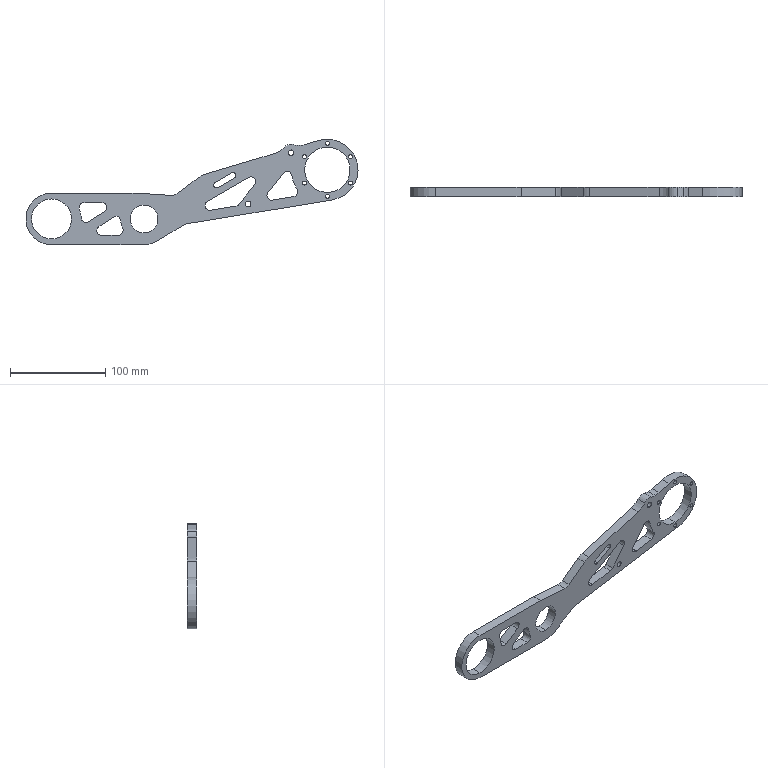Part | SolidWorks | features ICE 5, Fillet 2, Extrusion 1 | 1 solid | 74 faces | box 347.966 x 10 x 110.45 mm | volume 118705 mm3 | cylinder 53 | plane 21 | commonest cylinder face diameters 10 x15 4.2 x12 6 x7 40 x4 20 x2 29.15 x2